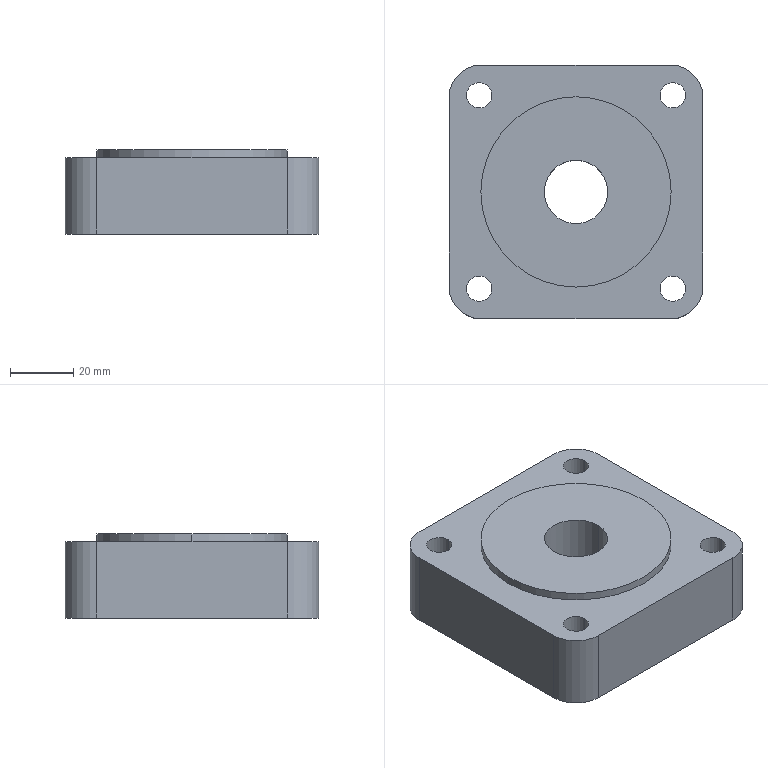Part | SolidWorks | features ICE 4, MirrorPattern 2, Extrusion 1, Fillet 1 | 1 solid | 32 faces | box 80 x 80 x 26.5 mm | volume 139825 mm3 | cylinder 20 | plane 12 | commonest cylinder face diameters 8 x8 20 x6 4 x4 60 x2
STEP:
#1=CARTESIAN_POINT('',(10.,0.,2.5));
#2=VERTEX_POINT('',#1);
#3=CARTESIAN_POINT('',(-10.,0.,2.5));
#4=VERTEX_POINT('',#3);
#5=CARTESIAN_POINT('',(0.,0.,2.5));
#6=DIRECTION('',(0.,0.,-1.));
#7=DIRECTION('',(1.,0.,0.));
#8=AXIS2_PLACEMENT_3D('',#5,#6,#7);
#9=CIRCLE('',#8,10.);
#10=EDGE_CURVE('',#2,#4,#9,.T.);
#11=ORIENTED_EDGE('',*,*,#10,.T.);
#12=CARTESIAN_POINT('',(-10.,0.,26.5));
#13=VERTEX_POINT('',#12);
#14=CARTESIAN_POINT('',(-10.,0.,-23.));
#15=DIRECTION('',(0.,0.,1.));
#16=VECTOR('',#15,1000.);
#17=LINE('',#14,#16);
#18=EDGE_CURVE('',#4,#13,#17,.T.);
#19=ORIENTED_EDGE('',*,*,#18,.T.);
#20=CARTESIAN_POINT('',(10.,0.,26.5));
#21=VERTEX_POINT('',#20);
#22=CARTESIAN_POINT('',(0.,0.,26.5));
#23=DIRECTION('',(0.,0.,1.));
#24=DIRECTION('',(1.,0.,0.));
#25=AXIS2_PLACEMENT_3D('',#22,#23,#24);
#26=CIRCLE('',#25,10.);
#27=EDGE_CURVE('',#13,#21,#26,.T.);
#28=ORIENTED_EDGE('',*,*,#27,.T.);
#29=CARTESIAN_POINT('',(10.,0.,-23.));
#30=DIRECTION('',(0.,0.,1.));
#31=VECTOR('',#30,1000.);
#32=LINE('',#29,#31);
#33=EDGE_CURVE('',#2,#21,#32,.T.);
#34=ORIENTED_EDGE('',*,*,#33,.F.);
#35=EDGE_LOOP('',(#11,#19,#28,#34));
#36=FACE_OUTER_BOUND('',#35,.T.);
#37=CARTESIAN_POINT('',(0.,0.,-23.));
#38=DIRECTION('',(0.,0.,1.));
#39=DIRECTION('',(1.,0.,0.));
#40=AXIS2_PLACEMENT_3D('',#37,#38,#39);
#41=CYLINDRICAL_SURFACE('',#40,10.);
#42=ADVANCED_FACE('',(#36),#41,.F.);
#43=CARTESIAN_POINT('',(30.,0.,26.5));
#44=VERTEX_POINT('',#43);
#45=CARTESIAN_POINT('',(-30.,0.,26.5));
#46=VERTEX_POINT('',#45);
#47=CARTESIAN_POINT('',(0.,0.,26.5));
#48=DIRECTION('',(0.,0.,1.));
#49=DIRECTION('',(1.,0.,0.));
#50=AXIS2_PLACEMENT_3D('',#47,#48,#49);
#51=CIRCLE('',#50,30.);
#52=EDGE_CURVE('',#44,#46,#51,.T.);
#53=ORIENTED_EDGE('',*,*,#52,.F.);
#54=CARTESIAN_POINT('',(30.,0.,24.));
#55=VERTEX_POINT('',#54);
#56=CARTESIAN_POINT('',(30.,0.,26.5));
#57=DIRECTION('',(0.,0.,-1.));
#58=VECTOR('',#57,1000.);
#59=LINE('',#56,#58);
#60=EDGE_CURVE('',#44,#55,#59,.T.);
#61=ORIENTED_EDGE('',*,*,#60,.T.);
#62=CARTESIAN_POINT('',(-30.,0.,24.));
#63=VERTEX_POINT('',#62);
#64=CARTESIAN_POINT('',(0.,0.,24.));
#65=DIRECTION('',(0.,0.,1.));
#66=DIRECTION('',(-1.,0.,0.));
#67=AXIS2_PLACEMENT_3D('',#64,#65,#66);
#68=CIRCLE('',#67,30.);
#69=EDGE_CURVE('',#55,#63,#68,.T.);
#70=ORIENTED_EDGE('',*,*,#69,.T.);
#71=CARTESIAN_POINT('',(-30.,0.,26.5));
#72=DIRECTION('',(0.,0.,-1.));
#73=VECTOR('',#72,1000.);
#74=LINE('',#71,#73);
#75=EDGE_CURVE('',#46,#63,#74,.T.);
#76=ORIENTED_EDGE('',*,*,#75,.F.);
#77=EDGE_LOOP('',(#53,#61,#70,#76));
#78=FACE_OUTER_BOUND('',#77,.T.);
#79=CARTESIAN_POINT('',(0.,0.,26.5));
#80=DIRECTION('',(0.,0.,-1.));
#81=DIRECTION('',(-1.,0.,0.));
#82=AXIS2_PLACEMENT_3D('',#79,#80,#81);
#83=CYLINDRICAL_SURFACE('',#82,30.);
#84=ADVANCED_FACE('',(#78),#83,.T.);
#85=CARTESIAN_POINT('',(34.5,30.5,0.));
#86=VERTEX_POINT('',#85);
#87=CARTESIAN_POINT('',(26.5,30.5,0.));
#88=VERTEX_POINT('',#87);
#89=CARTESIAN_POINT('',(30.5,30.5,0.));
#90=DIRECTION('',(0.,0.,-1.));
#91=DIRECTION('',(-1.,0.,0.));
#92=AXIS2_PLACEMENT_3D('',#89,#90,#91);
#93=CIRCLE('',#92,4.);
#94=EDGE_CURVE('',#86,#88,#93,.T.);
#95=ORIENTED_EDGE('',*,*,#94,.T.);
#96=CARTESIAN_POINT('',(26.5,30.5,24.));
#97=VERTEX_POINT('',#96);
#98=CARTESIAN_POINT('',(26.5,30.5,0.));
#99=DIRECTION('',(0.,0.,1.));
#100=VECTOR('',#99,1000.);
#101=LINE('',#98,#100);
#102=EDGE_CURVE('',#88,#97,#101,.T.);
#103=ORIENTED_EDGE('',*,*,#102,.T.);
#104=CARTESIAN_POINT('',(34.5,30.5,24.));
#105=VERTEX_POINT('',#104);
#106=CARTESIAN_POINT('',(30.5,30.5,24.));
#107=DIRECTION('',(0.,0.,1.));
#108=DIRECTION('',(-1.,0.,0.));
#109=AXIS2_PLACEMENT_3D('',#106,#107,#108);
#110=CIRCLE('',#109,4.);
#111=EDGE_CURVE('',#97,#105,#110,.T.);
#112=ORIENTED_EDGE('',*,*,#111,.T.);
#113=CARTESIAN_POINT('',(34.5,30.5,0.));
#114=DIRECTION('',(0.,0.,1.));
#115=VECTOR('',#114,1000.);
#116=LINE('',#113,#115);
#117=EDGE_CURVE('',#86,#105,#116,.T.);
#118=ORIENTED_EDGE('',*,*,#117,.F.);
#119=EDGE_LOOP('',(#95,#103,#112,#118));
#120=FACE_OUTER_BOUND('',#119,.T.);
#121=CARTESIAN_POINT('',(30.5,30.5,0.));
#122=DIRECTION('',(0.,0.,1.));
#123=DIRECTION('',(1.,0.,0.));
#124=AXIS2_PLACEMENT_3D('',#121,#122,#123);
#125=CYLINDRICAL_SURFACE('',#124,4.);
#126=ADVANCED_FACE('',(#120),#125,.F.);
#127=CARTESIAN_POINT('',(26.5,-30.5,0.));
#128=VERTEX_POINT('',#127);
#129=CARTESIAN_POINT('',(34.5,-30.5,0.));
#130=VERTEX_POINT('',#129);
#131=CARTESIAN_POINT('',(30.5,-30.5,0.));
#132=DIRECTION('',(0.,0.,1.));
#133=DIRECTION('',(-1.,0.,0.));
#134=AXIS2_PLACEMENT_3D('',#131,#132,#133);
#135=CIRCLE('',#134,4.);
#136=EDGE_CURVE('',#128,#130,#135,.T.);
#137=ORIENTED_EDGE('',*,*,#136,.F.);
#138=CARTESIAN_POINT('',(26.5,-30.5,24.));
#139=VERTEX_POINT('',#138);
#140=CARTESIAN_POINT('',(26.5,-30.5,0.));
#141=DIRECTION('',(0.,0.,1.));
#142=VECTOR('',#141,1000.);
#143=LINE('',#140,#142);
#144=EDGE_CURVE('',#128,#139,#143,.T.);
#145=ORIENTED_EDGE('',*,*,#144,.T.);
#146=CARTESIAN_POINT('',(34.5,-30.5,24.));
#147=VERTEX_POINT('',#146);
#148=CARTESIAN_POINT('',(30.5,-30.5,24.));
#149=DIRECTION('',(0.,0.,-1.));
#150=DIRECTION('',(-1.,0.,0.));
#151=AXIS2_PLACEMENT_3D('',#148,#149,#150);
#152=CIRCLE('',#151,4.);
#153=EDGE_CURVE('',#147,#139,#152,.T.);
#154=ORIENTED_EDGE('',*,*,#153,.F.);
#155=CARTESIAN_POINT('',(34.5,-30.5,0.));
#156=DIRECTION('',(0.,0.,1.));
#157=VECTOR('',#156,1000.);
#158=LINE('',#155,#157);
#159=EDGE_CURVE('',#130,#147,#158,.T.);
#160=ORIENTED_EDGE('',*,*,#159,.F.);
#161=EDGE_LOOP('',(#137,#145,#154,#160));
#162=FACE_OUTER_BOUND('',#161,.T.);
#163=CARTESIAN_POINT('',(30.5,-30.5,0.));
#164=DIRECTION('',(0.,0.,1.));
#165=DIRECTION('',(1.,0.,0.));
#166=AXIS2_PLACEMENT_3D('',#163,#164,#165);
#167=CYLINDRICAL_SURFACE('',#166,4.);
#168=ADVANCED_FACE('',(#162),#167,.F.);
#169=CARTESIAN_POINT('',(-26.5,-30.5,0.));
#170=VERTEX_POINT('',#169);
#171=CARTESIAN_POINT('',(-34.5,-30.5,0.));
#172=VERTEX_POINT('',#171);
#173=CARTESIAN_POINT('',(-30.5,-30.5,0.));
#174=DIRECTION('',(0.,0.,-1.));
#175=DIRECTION('',(1.,0.,0.));
#176=AXIS2_PLACEMENT_3D('',#173,#174,#175);
#177=CIRCLE('',#176,4.);
#178=EDGE_CURVE('',#170,#172,#177,.T.);
#179=ORIENTED_EDGE('',*,*,#178,.T.);
#180=CARTESIAN_POINT('',(-34.5,-30.5,24.));
#181=VERTEX_POINT('',#180);
#182=CARTESIAN_POINT('',(-34.5,-30.5,0.));
#183=DIRECTION('',(0.,0.,1.));
#184=VECTOR('',#183,1000.);
#185=LINE('',#182,#184);
#186=EDGE_CURVE('',#172,#181,#185,.T.);
#187=ORIENTED_EDGE('',*,*,#186,.T.);
#188=CARTESIAN_POINT('',(-26.5,-30.5,24.));
#189=VERTEX_POINT('',#188);
#190=CARTESIAN_POINT('',(-30.5,-30.5,24.));
#191=DIRECTION('',(0.,0.,1.));
#192=DIRECTION('',(-1.,0.,0.));
#193=AXIS2_PLACEMENT_3D('',#190,#191,#192);
#194=CIRCLE('',#193,4.);
#195=EDGE_CURVE('',#181,#189,#194,.T.);
#196=ORIENTED_EDGE('',*,*,#195,.T.);
#197=CARTESIAN_POINT('',(-26.5,-30.5,0.));
#198=DIRECTION('',(0.,0.,1.));
#199=VECTOR('',#198,1000.);
#200=LINE('',#197,#199);
#201=EDGE_CURVE('',#170,#189,#200,.T.);
#202=ORIENTED_EDGE('',*,*,#201,.F.);
#203=EDGE_LOOP('',(#179,#187,#196,#202));
#204=FACE_OUTER_BOUND('',#203,.T.);
#205=CARTESIAN_POINT('',(-30.5,-30.5,0.));
#206=DIRECTION('',(0.,0.,1.));
#207=DIRECTION('',(1.,0.,0.));
#208=AXIS2_PLACEMENT_3D('',#205,#206,#207);
#209=CYLINDRICAL_SURFACE('',#208,4.);
#210=ADVANCED_FACE('',(#204),#209,.F.);
#211=CARTESIAN_POINT('',(-34.5,30.5,0.));
#212=VERTEX_POINT('',#211);
#213=CARTESIAN_POINT('',(-26.5,30.5,0.));
#214=VERTEX_POINT('',#213);
#215=CARTESIAN_POINT('',(-30.5,30.5,0.));
#216=DIRECTION('',(0.,0.,1.));
#217=DIRECTION('',(1.,0.,0.));
#218=AXIS2_PLACEMENT_3D('',#215,#216,#217);
#219=CIRCLE('',#218,4.);
#220=EDGE_CURVE('',#212,#214,#219,.T.);
#221=ORIENTED_EDGE('',*,*,#220,.F.);
#222=CARTESIAN_POINT('',(-34.5,30.5,24.));
#223=VERTEX_POINT('',#222);
#224=CARTESIAN_POINT('',(-34.5,30.5,0.));
#225=DIRECTION('',(0.,0.,1.));
#226=VECTOR('',#225,1000.);
#227=LINE('',#224,#226);
#228=EDGE_CURVE('',#212,#223,#227,.T.);
#229=ORIENTED_EDGE('',*,*,#228,.T.);
#230=CARTESIAN_POINT('',(-26.5,30.5,24.));
#231=VERTEX_POINT('',#230);
#232=CARTESIAN_POINT('',(-30.5,30.5,24.));
#233=DIRECTION('',(0.,0.,-1.));
#234=DIRECTION('',(-1.,0.,0.));
#235=AXIS2_PLACEMENT_3D('',#232,#233,#234);
#236=CIRCLE('',#235,4.);
#237=EDGE_CURVE('',#231,#223,#236,.T.);
#238=ORIENTED_EDGE('',*,*,#237,.F.);
#239=CARTESIAN_POINT('',(-26.5,30.5,0.));
#240=DIRECTION('',(0.,0.,1.));
#241=VECTOR('',#240,1000.);
#242=LINE('',#239,#241);
#243=EDGE_CURVE('',#214,#231,#242,.T.);
#244=ORIENTED_EDGE('',*,*,#243,.F.);
#245=EDGE_LOOP('',(#221,#229,#238,#244));
#246=FACE_OUTER_BOUND('',#245,.T.);
#247=CARTESIAN_POINT('',(-30.5,30.5,0.));
#248=DIRECTION('',(0.,0.,1.));
#249=DIRECTION('',(1.,0.,0.));
#250=AXIS2_PLACEMENT_3D('',#247,#248,#249);
#251=CYLINDRICAL_SURFACE('',#250,4.);
#252=ADVANCED_FACE('',(#246),#251,.F.);
#253=CARTESIAN_POINT('',(40.,-30.,24.));
#254=VERTEX_POINT('',#253);
#255=CARTESIAN_POINT('',(40.,30.,24.));
#256=VERTEX_POINT('',#255);
#257=CARTESIAN_POINT('',(40.,-40.,24.));
#258=DIRECTION('',(0.,1.,0.));
#259=VECTOR('',#258,1000.);
#260=LINE('',#257,#259);
#261=EDGE_CURVE('',#254,#256,#260,.T.);
#262=ORIENTED_EDGE('',*,*,#261,.F.);
#263=CARTESIAN_POINT('',(40.,-30.,0.));
#264=VERTEX_POINT('',#263);
#265=CARTESIAN_POINT('',(40.,-30.,24.));
#266=DIRECTION('',(0.,0.,-1.));
#267=VECTOR('',#266,1000.);
#268=LINE('',#265,#267);
#269=EDGE_CURVE('',#254,#264,#268,.T.);
#270=ORIENTED_EDGE('',*,*,#269,.T.);
#271=CARTESIAN_POINT('',(40.,30.,0.));
#272=VERTEX_POINT('',#271);
#273=CARTESIAN_POINT('',(40.,-40.,0.));
#274=DIRECTION('',(0.,1.,0.));
#275=VECTOR('',#274,1000.);
#276=LINE('',#273,#275);
#277=EDGE_CURVE('',#264,#272,#276,.T.);
#278=ORIENTED_EDGE('',*,*,#277,.T.);
#279=CARTESIAN_POINT('',(40.,30.,24.));
#280=DIRECTION('',(0.,0.,1.));
#281=VECTOR('',#280,1000.);
#282=LINE('',#279,#281);
#283=EDGE_CURVE('',#272,#256,#282,.T.);
#284=ORIENTED_EDGE('',*,*,#283,.T.);
#285=EDGE_LOOP('',(#262,#270,#278,#284));
#286=FACE_OUTER_BOUND('',#285,.T.);
#287=CARTESIAN_POINT('',(40.,-40.,24.));
#288=DIRECTION('',(-1.,0.,0.));
#289=DIRECTION('',(0.,0.,1.));
#290=AXIS2_PLACEMENT_3D('',#287,#288,#289);
#291=PLANE('',#290);
#292=ADVANCED_FACE('',(#286),#291,.F.);
#293=CARTESIAN_POINT('',(30.,40.,24.));
#294=VERTEX_POINT('',#293);
#295=CARTESIAN_POINT('',(-30.,40.,24.));
#296=VERTEX_POINT('',#295);
#297=CARTESIAN_POINT('',(-40.,40.,24.));
#298=DIRECTION('',(-1.,0.,0.));
#299=VECTOR('',#298,1000.);
#300=LINE('',#297,#299);
#301=EDGE_CURVE('',#294,#296,#300,.T.);
#302=ORIENTED_EDGE('',*,*,#301,.F.);
#303=CARTESIAN_POINT('',(30.,40.,0.));
#304=VERTEX_POINT('',#303);
#305=CARTESIAN_POINT('',(30.,40.,24.));
#306=DIRECTION('',(0.,0.,-1.));
#307=VECTOR('',#306,1000.);
#308=LINE('',#305,#307);
#309=EDGE_CURVE('',#294,#304,#308,.T.);
#310=ORIENTED_EDGE('',*,*,#309,.T.);
#311=CARTESIAN_POINT('',(-30.,40.,0.));
#312=VERTEX_POINT('',#311);
#313=CARTESIAN_POINT('',(-40.,40.,0.));
#314=DIRECTION('',(-1.,0.,0.));
#315=VECTOR('',#314,1000.);
#316=LINE('',#313,#315);
#317=EDGE_CURVE('',#304,#312,#316,.T.);
#318=ORIENTED_EDGE('',*,*,#317,.T.);
#319=CARTESIAN_POINT('',(-30.,40.,24.));
#320=DIRECTION('',(0.,0.,1.));
#321=VECTOR('',#320,1000.);
#322=LINE('',#319,#321);
#323=EDGE_CURVE('',#312,#296,#322,.T.);
#324=ORIENTED_EDGE('',*,*,#323,.T.);
#325=EDGE_LOOP('',(#302,#310,#318,#324));
#326=FACE_OUTER_BOUND('',#325,.T.);
#327=CARTESIAN_POINT('',(-40.,40.,24.));
#328=DIRECTION('',(0.,-1.,0.));
#329=DIRECTION('',(0.,0.,-1.));
#330=AXIS2_PLACEMENT_3D('',#327,#328,#329);
#331=PLANE('',#330);
#332=ADVANCED_FACE('',(#326),#331,.F.);
#333=CARTESIAN_POINT('',(-40.,30.,0.));
#334=VERTEX_POINT('',#333);
#335=CARTESIAN_POINT('',(-40.,-30.,0.));
#336=VERTEX_POINT('',#335);
#337=CARTESIAN_POINT('',(-40.,-40.,0.));
#338=DIRECTION('',(0.,-1.,0.));
#339=VECTOR('',#338,1000.);
#340=LINE('',#337,#339);
#341=EDGE_CURVE('',#334,#336,#340,.T.);
#342=ORIENTED_EDGE('',*,*,#341,.T.);
#343=CARTESIAN_POINT('',(-40.,-30.,24.));
#344=VERTEX_POINT('',#343);
#345=CARTESIAN_POINT('',(-40.,-30.,24.));
#346=DIRECTION('',(0.,0.,1.));
#347=VECTOR('',#346,1000.);
#348=LINE('',#345,#347);
#349=EDGE_CURVE('',#336,#344,#348,.T.);
#350=ORIENTED_EDGE('',*,*,#349,.T.);
#351=CARTESIAN_POINT('',(-40.,30.,24.));
#352=VERTEX_POINT('',#351);
#353=CARTESIAN_POINT('',(-40.,-40.,24.));
#354=DIRECTION('',(0.,-1.,0.));
#355=VECTOR('',#354,1000.);
#356=LINE('',#353,#355);
#357=EDGE_CURVE('',#352,#344,#356,.T.);
#358=ORIENTED_EDGE('',*,*,#357,.F.);
#359=CARTESIAN_POINT('',(-40.,30.,24.));
#360=DIRECTION('',(0.,0.,-1.));
#361=VECTOR('',#360,1000.);
#362=LINE('',#359,#361);
#363=EDGE_CURVE('',#352,#334,#362,.T.);
#364=ORIENTED_EDGE('',*,*,#363,.T.);
#365=EDGE_LOOP('',(#342,#350,#358,#364));
#366=FACE_OUTER_BOUND('',#365,.T.);
#367=CARTESIAN_POINT('',(-40.,-40.,24.));
#368=DIRECTION('',(1.,0.,0.));
#369=DIRECTION('',(0.,0.,-1.));
#370=AXIS2_PLACEMENT_3D('',#367,#368,#369);
#371=PLANE('',#370);
#372=ADVANCED_FACE('',(#366),#371,.F.);
#373=CARTESIAN_POINT('',(-30.,-40.,24.));
#374=VERTEX_POINT('',#373);
#375=CARTESIAN_POINT('',(30.,-40.,24.));
#376=VERTEX_POINT('',#375);
#377=CARTESIAN_POINT('',(-40.,-40.,24.));
#378=DIRECTION('',(1.,0.,0.));
#379=VECTOR('',#378,1000.);
#380=LINE('',#377,#379);
#381=EDGE_CURVE('',#374,#376,#380,.T.);
#382=ORIENTED_EDGE('',*,*,#381,.F.);
#383=CARTESIAN_POINT('',(-30.,-40.,0.));
#384=VERTEX_POINT('',#383);
#385=CARTESIAN_POINT('',(-30.,-40.,24.));
#386=DIRECTION('',(0.,0.,-1.));
#387=VECTOR('',#386,1000.);
#388=LINE('',#385,#387);
#389=EDGE_CURVE('',#374,#384,#388,.T.);
#390=ORIENTED_EDGE('',*,*,#389,.T.);
#391=CARTESIAN_POINT('',(30.,-40.,0.));
#392=VERTEX_POINT('',#391);
#393=CARTESIAN_POINT('',(-40.,-40.,0.));
#394=DIRECTION('',(1.,0.,0.));
#395=VECTOR('',#394,1000.);
#396=LINE('',#393,#395);
#397=EDGE_CURVE('',#384,#392,#396,.T.);
#398=ORIENTED_EDGE('',*,*,#397,.T.);
#399=CARTESIAN_POINT('',(30.,-40.,24.));
#400=DIRECTION('',(0.,0.,1.));
#401=VECTOR('',#400,1000.);
#402=LINE('',#399,#401);
#403=EDGE_CURVE('',#392,#376,#402,.T.);
#404=ORIENTED_EDGE('',*,*,#403,.T.);
#405=EDGE_LOOP('',(#382,#390,#398,#404));
#406=FACE_OUTER_BOUND('',#405,.T.);
#407=CARTESIAN_POINT('',(-40.,-40.,24.));
#408=DIRECTION('',(0.,1.,0.));
#409=DIRECTION('',(0.,0.,1.));
#410=AXIS2_PLACEMENT_3D('',#407,#408,#409);
#411=PLANE('',#410);
#412=ADVANCED_FACE('',(#406),#411,.F.);
#413=CARTESIAN_POINT('',(0.,0.,24.));
#414=DIRECTION('',(0.,0.,1.));
#415=DIRECTION('',(-1.,0.,0.));
#416=AXIS2_PLACEMENT_3D('',#413,#414,#415);
#417=CIRCLE('',#416,30.);
#418=EDGE_CURVE('',#63,#55,#417,.T.);
#419=ORIENTED_EDGE('',*,*,#418,.F.);
#420=ORIENTED_EDGE('',*,*,#69,.F.);
#421=EDGE_LOOP('',(#419,#420));
#422=FACE_BOUND('',#421,.T.);
#423=CARTESIAN_POINT('',(30.5,30.5,24.));
#424=DIRECTION('',(0.,0.,1.));
#425=DIRECTION('',(-1.,0.,0.));
#426=AXIS2_PLACEMENT_3D('',#423,#424,#425);
#427=CIRCLE('',#426,4.);
#428=EDGE_CURVE('',#105,#97,#427,.T.);
#429=ORIENTED_EDGE('',*,*,#428,.F.);
#430=ORIENTED_EDGE('',*,*,#111,.F.);
#431=EDGE_LOOP('',(#429,#430));
#432=FACE_BOUND('',#431,.T.);
#433=ORIENTED_EDGE('',*,*,#153,.T.);
#434=CARTESIAN_POINT('',(30.5,-30.5,24.));
#435=DIRECTION('',(0.,0.,-1.));
#436=DIRECTION('',(-1.,0.,0.));
#437=AXIS2_PLACEMENT_3D('',#434,#435,#436);
#438=CIRCLE('',#437,4.);
#439=EDGE_CURVE('',#139,#147,#438,.T.);
#440=ORIENTED_EDGE('',*,*,#439,.T.);
#441=EDGE_LOOP('',(#433,#440));
#442=FACE_BOUND('',#441,.T.);
#443=CARTESIAN_POINT('',(-30.5,-30.5,24.));
#444=DIRECTION('',(0.,0.,1.));
#445=DIRECTION('',(-1.,0.,0.));
#446=AXIS2_PLACEMENT_3D('',#443,#444,#445);
#447=CIRCLE('',#446,4.);
#448=EDGE_CURVE('',#189,#181,#447,.T.);
#449=ORIENTED_EDGE('',*,*,#448,.F.);
#450=ORIENTED_EDGE('',*,*,#195,.F.);
#451=EDGE_LOOP('',(#449,#450));
#452=FACE_BOUND('',#451,.T.);
#453=ORIENTED_EDGE('',*,*,#237,.T.);
#454=CARTESIAN_POINT('',(-30.5,30.5,24.));
#455=DIRECTION('',(0.,0.,-1.));
#456=DIRECTION('',(-1.,0.,0.));
#457=AXIS2_PLACEMENT_3D('',#454,#455,#456);
#458=CIRCLE('',#457,4.);
#459=EDGE_CURVE('',#223,#231,#458,.T.);
#460=ORIENTED_EDGE('',*,*,#459,.T.);
#461=EDGE_LOOP('',(#453,#460));
#462=FACE_BOUND('',#461,.T.);
#463=ORIENTED_EDGE('',*,*,#357,.T.);
#464=CARTESIAN_POINT('',(-30.,-30.,24.));
#465=DIRECTION('',(0.,0.,1.));
#466=DIRECTION('',(-1.,0.,0.));
#467=AXIS2_PLACEMENT_3D('',#464,#465,#466);
#468=CIRCLE('',#467,10.);
#469=EDGE_CURVE('',#344,#374,#468,.T.);
#470=ORIENTED_EDGE('',*,*,#469,.T.);
#471=ORIENTED_EDGE('',*,*,#381,.T.);
#472=CARTESIAN_POINT('',(30.,-30.,24.));
#473=DIRECTION('',(0.,0.,1.));
#474=DIRECTION('',(-1.,0.,0.));
#475=AXIS2_PLACEMENT_3D('',#472,#473,#474);
#476=CIRCLE('',#475,10.);
#477=EDGE_CURVE('',#376,#254,#476,.T.);
#478=ORIENTED_EDGE('',*,*,#477,.T.);
#479=ORIENTED_EDGE('',*,*,#261,.T.);
#480=CARTESIAN_POINT('',(30.,30.,24.));
#481=DIRECTION('',(0.,0.,1.));
#482=DIRECTION('',(-1.,0.,0.));
#483=AXIS2_PLACEMENT_3D('',#480,#481,#482);
#484=CIRCLE('',#483,10.);
#485=EDGE_CURVE('',#256,#294,#484,.T.);
#486=ORIENTED_EDGE('',*,*,#485,.T.);
#487=ORIENTED_EDGE('',*,*,#301,.T.);
#488=CARTESIAN_POINT('',(-30.,30.,24.));
#489=DIRECTION('',(0.,0.,1.));
#490=DIRECTION('',(-1.,0.,0.));
#491=AXIS2_PLACEMENT_3D('',#488,#489,#490);
#492=CIRCLE('',#491,10.);
#493=EDGE_CURVE('',#296,#352,#492,.T.);
#494=ORIENTED_EDGE('',*,*,#493,.T.);
#495=EDGE_LOOP('',(#463,#470,#471,#478,#479,#486,#487,#494));
#496=FACE_OUTER_BOUND('',#495,.T.);
#497=CARTESIAN_POINT('',(0.,0.,24.));
#498=DIRECTION('',(0.,0.,-1.));
#499=DIRECTION('',(-1.,0.,0.));
#500=AXIS2_PLACEMENT_3D('',#497,#498,#499);
#501=PLANE('',#500);
#502=ADVANCED_FACE('',(#422,#432,#442,#452,#462,#496),#501,.F.);
#503=CARTESIAN_POINT('',(25.263,-23.439,0.));
#504=VERTEX_POINT('',#503);
#505=CARTESIAN_POINT('',(23.263,-25.439,0.));
#506=VERTEX_POINT('',#505);
#507=CARTESIAN_POINT('',(23.263,-23.439,0.));
#508=DIRECTION('',(0.,0.,-1.));
#509=DIRECTION('',(1.,0.,0.));
#510=AXIS2_PLACEMENT_3D('',#507,#508,#509);
#511=CIRCLE('',#510,2.);
#512=EDGE_CURVE('',#504,#506,#511,.T.);
#513=ORIENTED_EDGE('',*,*,#512,.F.);
#514=CARTESIAN_POINT('',(25.263,23.439,0.));
#515=VERTEX_POINT('',#514);
#516=CARTESIAN_POINT('',(25.263,-23.439,0.));
#517=DIRECTION('',(0.,-1.,0.));
#518=VECTOR('',#517,1000.);
#519=LINE('',#516,#518);
#520=EDGE_CURVE('',#515,#504,#519,.T.);
#521=ORIENTED_EDGE('',*,*,#520,.F.);
#522=CARTESIAN_POINT('',(23.263,25.439,0.));
#523=VERTEX_POINT('',#522);
#524=CARTESIAN_POINT('',(23.263,23.439,0.));
#525=DIRECTION('',(0.,0.,-1.));
#526=DIRECTION('',(1.,0.,0.));
#527=AXIS2_PLACEMENT_3D('',#524,#525,#526);
#528=CIRCLE('',#527,2.);
#529=EDGE_CURVE('',#523,#515,#528,.T.);
#530=ORIENTED_EDGE('',*,*,#529,.F.);
#531=CARTESIAN_POINT('',(-23.263,25.439,0.));
#532=VERTEX_POINT('',#531);
#533=CARTESIAN_POINT('',(23.263,25.439,0.));
#534=DIRECTION('',(1.,0.,0.));
#535=VECTOR('',#534,1000.);
#536=LINE('',#533,#535);
#537=EDGE_CURVE('',#532,#523,#536,.T.);
#538=ORIENTED_EDGE('',*,*,#537,.F.);
#539=CARTESIAN_POINT('',(-25.263,23.439,0.));
#540=VERTEX_POINT('',#539);
#541=CARTESIAN_POINT('',(-23.263,23.439,0.));
#542=DIRECTION('',(0.,0.,-1.));
#543=DIRECTION('',(-1.,0.,0.));
#544=AXIS2_PLACEMENT_3D('',#541,#542,#543);
#545=CIRCLE('',#544,2.);
#546=EDGE_CURVE('',#540,#532,#545,.T.);
#547=ORIENTED_EDGE('',*,*,#546,.F.);
#548=CARTESIAN_POINT('',(-25.263,-23.439,0.));
#549=VERTEX_POINT('',#548);
#550=CARTESIAN_POINT('',(-25.263,-23.439,0.));
#551=DIRECTION('',(0.,1.,0.));
#552=VECTOR('',#551,1000.);
#553=LINE('',#550,#552);
#554=EDGE_CURVE('',#549,#540,#553,.T.);
#555=ORIENTED_EDGE('',*,*,#554,.F.);
#556=CARTESIAN_POINT('',(-23.263,-25.439,0.));
#557=VERTEX_POINT('',#556);
#558=CARTESIAN_POINT('',(-23.263,-23.439,0.));
#559=DIRECTION('',(0.,0.,-1.));
#560=DIRECTION('',(1.,0.,0.));
#561=AXIS2_PLACEMENT_3D('',#558,#559,#560);
#562=CIRCLE('',#561,2.);
#563=EDGE_CURVE('',#557,#549,#562,.T.);
#564=ORIENTED_EDGE('',*,*,#563,.F.);
#565=CARTESIAN_POINT('',(23.263,-25.439,0.));
#566=DIRECTION('',(-1.,0.,0.));
#567=VECTOR('',#566,1000.);
#568=LINE('',#565,#567);
#569=EDGE_CURVE('',#506,#557,#568,.T.);
#570=ORIENTED_EDGE('',*,*,#569,.F.);
#571=EDGE_LOOP('',(#513,#521,#530,#538,#547,#555,#564,#570));
#572=FACE_BOUND('',#571,.T.);
#573=ORIENTED_EDGE('',*,*,#94,.F.);
#574=CARTESIAN_POINT('',(30.5,30.5,0.));
#575=DIRECTION('',(0.,0.,-1.));
#576=DIRECTION('',(-1.,0.,0.));
#577=AXIS2_PLACEMENT_3D('',#574,#575,#576);
#578=CIRCLE('',#577,4.);
#579=EDGE_CURVE('',#88,#86,#578,.T.);
#580=ORIENTED_EDGE('',*,*,#579,.F.);
#581=EDGE_LOOP('',(#573,#580));
#582=FACE_BOUND('',#581,.T.);
#583=CARTESIAN_POINT('',(30.5,-30.5,0.));
#584=DIRECTION('',(0.,0.,1.));
#585=DIRECTION('',(-1.,0.,0.));
#586=AXIS2_PLACEMENT_3D('',#583,#584,#585);
#587=CIRCLE('',#586,4.);
#588=EDGE_CURVE('',#130,#128,#587,.T.);
#589=ORIENTED_EDGE('',*,*,#588,.T.);
#590=ORIENTED_EDGE('',*,*,#136,.T.);
#591=EDGE_LOOP('',(#589,#590));
#592=FACE_BOUND('',#591,.T.);
#593=ORIENTED_EDGE('',*,*,#178,.F.);
#594=CARTESIAN_POINT('',(-30.5,-30.5,0.));
#595=DIRECTION('',(0.,0.,-1.));
#596=DIRECTION('',(1.,0.,0.));
#597=AXIS2_PLACEMENT_3D('',#594,#595,#596);
#598=CIRCLE('',#597,4.);
#599=EDGE_CURVE('',#172,#170,#598,.T.);
#600=ORIENTED_EDGE('',*,*,#599,.F.);
#601=EDGE_LOOP('',(#593,#600));
#602=FACE_BOUND('',#601,.T.);
#603=CARTESIAN_POINT('',(-30.5,30.5,0.));
#604=DIRECTION('',(0.,0.,1.));
#605=DIRECTION('',(1.,0.,0.));
#606=AXIS2_PLACEMENT_3D('',#603,#604,#605);
#607=CIRCLE('',#606,4.);
#608=EDGE_CURVE('',#214,#212,#607,.T.);
#609=ORIENTED_EDGE('',*,*,#608,.T.);
#610=ORIENTED_EDGE('',*,*,#220,.T.);
#611=EDGE_LOOP('',(#609,#610));
#612=FACE_BOUND('',#611,.T.);
#613=ORIENTED_EDGE('',*,*,#397,.F.);
#614=CARTESIAN_POINT('',(-30.,-30.,0.));
#615=DIRECTION('',(0.,0.,-1.));
#616=DIRECTION('',(-1.,0.,0.));
#617=AXIS2_PLACEMENT_3D('',#614,#615,#616);
#618=CIRCLE('',#617,10.);
#619=EDGE_CURVE('',#384,#336,#618,.T.);
#620=ORIENTED_EDGE('',*,*,#619,.T.);
#621=ORIENTED_EDGE('',*,*,#341,.F.);
#622=CARTESIAN_POINT('',(-30.,30.,0.));
#623=DIRECTION('',(0.,0.,-1.));
#624=DIRECTION('',(-1.,0.,0.));
#625=AXIS2_PLACEMENT_3D('',#622,#623,#624);
#626=CIRCLE('',#625,10.);
#627=EDGE_CURVE('',#334,#312,#626,.T.);
#628=ORIENTED_EDGE('',*,*,#627,.T.);
#629=ORIENTED_EDGE('',*,*,#317,.F.);
#630=CARTESIAN_POINT('',(30.,30.,0.));
#631=DIRECTION('',(0.,0.,-1.));
#632=DIRECTION('',(-1.,0.,0.));
#633=AXIS2_PLACEMENT_3D('',#630,#631,#632);
#634=CIRCLE('',#633,10.);
#635=EDGE_CURVE('',#304,#272,#634,.T.);
#636=ORIENTED_EDGE('',*,*,#635,.T.);
#637=ORIENTED_EDGE('',*,*,#277,.F.);
#638=CARTESIAN_POINT('',(30.,-30.,0.));
#639=DIRECTION('',(0.,0.,-1.));
#640=DIRECTION('',(-1.,0.,0.));
#641=AXIS2_PLACEMENT_3D('',#638,#639,#640);
#642=CIRCLE('',#641,10.);
#643=EDGE_CURVE('',#264,#392,#642,.T.);
#644=ORIENTED_EDGE('',*,*,#643,.T.);
#645=EDGE_LOOP('',(#613,#620,#621,#628,#629,#636,#637,#644));
#646=FACE_OUTER_BOUND('',#645,.T.);
#647=CARTESIAN_POINT('',(0.,0.,0.));
#648=DIRECTION('',(0.,0.,-1.));
#649=DIRECTION('',(-1.,0.,0.));
#650=AXIS2_PLACEMENT_3D('',#647,#648,#649);
#651=PLANE('',#650);
#652=ADVANCED_FACE('',(#572,#582,#592,#602,#612,#646),#651,.T.);
#653=ORIENTED_EDGE('',*,*,#469,.F.);
#654=ORIENTED_EDGE('',*,*,#349,.F.);
#655=ORIENTED_EDGE('',*,*,#619,.F.);
#656=ORIENTED_EDGE('',*,*,#389,.F.);
#657=EDGE_LOOP('',(#653,#654,#655,#656));
#658=FACE_OUTER_BOUND('',#657,.T.);
#659=CARTESIAN_POINT('',(-30.,-30.,24.));
#660=DIRECTION('',(0.,0.,-1.));
#661=DIRECTION('',(-1.,0.,0.));
#662=AXIS2_PLACEMENT_3D('',#659,#660,#661);
#663=CYLINDRICAL_SURFACE('',#662,10.);
#664=ADVANCED_FACE('',(#658),#663,.T.);
#665=ORIENTED_EDGE('',*,*,#477,.F.);
#666=ORIENTED_EDGE('',*,*,#403,.F.);
#667=ORIENTED_EDGE('',*,*,#643,.F.);
#668=ORIENTED_EDGE('',*,*,#269,.F.);
#669=EDGE_LOOP('',(#665,#666,#667,#668));
#670=FACE_OUTER_BOUND('',#669,.T.);
#671=CARTESIAN_POINT('',(30.,-30.,24.));
#672=DIRECTION('',(0.,0.,-1.));
#673=DIRECTION('',(-1.,0.,0.));
#674=AXIS2_PLACEMENT_3D('',#671,#672,#673);
#675=CYLINDRICAL_SURFACE('',#674,10.);
#676=ADVANCED_FACE('',(#670),#675,.T.);
#677=ORIENTED_EDGE('',*,*,#485,.F.);
#678=ORIENTED_EDGE('',*,*,#283,.F.);
#679=ORIENTED_EDGE('',*,*,#635,.F.);
#680=ORIENTED_EDGE('',*,*,#309,.F.);
#681=EDGE_LOOP('',(#677,#678,#679,#680));
#682=FACE_OUTER_BOUND('',#681,.T.);
#683=CARTESIAN_POINT('',(30.,30.,24.));
#684=DIRECTION('',(0.,0.,-1.));
#685=DIRECTION('',(-1.,0.,0.));
#686=AXIS2_PLACEMENT_3D('',#683,#684,#685);
#687=CYLINDRICAL_SURFACE('',#686,10.);
#688=ADVANCED_FACE('',(#682),#687,.T.);
#689=ORIENTED_EDGE('',*,*,#493,.F.);
#690=ORIENTED_EDGE('',*,*,#323,.F.);
#691=ORIENTED_EDGE('',*,*,#627,.F.);
#692=ORIENTED_EDGE('',*,*,#363,.F.);
#693=EDGE_LOOP('',(#689,#690,#691,#692));
#694=FACE_OUTER_BOUND('',#693,.T.);
#695=CARTESIAN_POINT('',(-30.,30.,24.));
#696=DIRECTION('',(0.,0.,-1.));
#697=DIRECTION('',(-1.,0.,0.));
#698=AXIS2_PLACEMENT_3D('',#695,#696,#697);
#699=CYLINDRICAL_SURFACE('',#698,10.);
#700=ADVANCED_FACE('',(#694),#699,.T.);
#701=ORIENTED_EDGE('',*,*,#228,.F.);
#702=ORIENTED_EDGE('',*,*,#608,.F.);
#703=ORIENTED_EDGE('',*,*,#243,.T.);
#704=ORIENTED_EDGE('',*,*,#459,.F.);
#705=EDGE_LOOP('',(#701,#702,#703,#704));
#706=FACE_OUTER_BOUND('',#705,.T.);
#707=CARTESIAN_POINT('',(-30.5,30.5,0.));
#708=DIRECTION('',(0.,0.,1.));
#709=DIRECTION('',(1.,0.,0.));
#710=AXIS2_PLACEMENT_3D('',#707,#708,#709);
#711=CYLINDRICAL_SURFACE('',#710,4.);
#712=ADVANCED_FACE('',(#706),#711,.F.);
#713=ORIENTED_EDGE('',*,*,#186,.F.);
#714=ORIENTED_EDGE('',*,*,#599,.T.);
#715=ORIENTED_EDGE('',*,*,#201,.T.);
#716=ORIENTED_EDGE('',*,*,#448,.T.);
#717=EDGE_LOOP('',(#713,#714,#715,#716));
#718=FACE_OUTER_BOUND('',#717,.T.);
#719=CARTESIAN_POINT('',(-30.5,-30.5,0.));
#720=DIRECTION('',(0.,0.,1.));
#721=DIRECTION('',(1.,0.,0.));
#722=AXIS2_PLACEMENT_3D('',#719,#720,#721);
#723=CYLINDRICAL_SURFACE('',#722,4.);
#724=ADVANCED_FACE('',(#718),#723,.F.);
#725=ORIENTED_EDGE('',*,*,#144,.F.);
#726=ORIENTED_EDGE('',*,*,#588,.F.);
#727=ORIENTED_EDGE('',*,*,#159,.T.);
#728=ORIENTED_EDGE('',*,*,#439,.F.);
#729=EDGE_LOOP('',(#725,#726,#727,#728));
#730=FACE_OUTER_BOUND('',#729,.T.);
#731=CARTESIAN_POINT('',(30.5,-30.5,0.));
#732=DIRECTION('',(0.,0.,1.));
#733=DIRECTION('',(1.,0.,0.));
#734=AXIS2_PLACEMENT_3D('',#731,#732,#733);
#735=CYLINDRICAL_SURFACE('',#734,4.);
#736=ADVANCED_FACE('',(#730),#735,.F.);
#737=ORIENTED_EDGE('',*,*,#102,.F.);
#738=ORIENTED_EDGE('',*,*,#579,.T.);
#739=ORIENTED_EDGE('',*,*,#117,.T.);
#740=ORIENTED_EDGE('',*,*,#428,.T.);
#741=EDGE_LOOP('',(#737,#738,#739,#740));
#742=FACE_OUTER_BOUND('',#741,.T.);
#743=CARTESIAN_POINT('',(30.5,30.5,0.));
#744=DIRECTION('',(0.,0.,1.));
#745=DIRECTION('',(1.,0.,0.));
#746=AXIS2_PLACEMENT_3D('',#743,#744,#745);
#747=CYLINDRICAL_SURFACE('',#746,4.);
#748=ADVANCED_FACE('',(#742),#747,.F.);
#749=ORIENTED_EDGE('',*,*,#60,.F.);
#750=CARTESIAN_POINT('',(0.,0.,26.5));
#751=DIRECTION('',(0.,0.,1.));
#752=DIRECTION('',(1.,0.,0.));
#753=AXIS2_PLACEMENT_3D('',#750,#751,#752);
#754=CIRCLE('',#753,30.);
#755=EDGE_CURVE('',#46,#44,#754,.T.);
#756=ORIENTED_EDGE('',*,*,#755,.F.);
#757=ORIENTED_EDGE('',*,*,#75,.T.);
#758=ORIENTED_EDGE('',*,*,#418,.T.);
#759=EDGE_LOOP('',(#749,#756,#757,#758));
#760=FACE_OUTER_BOUND('',#759,.T.);
#761=CARTESIAN_POINT('',(0.,0.,26.5));
#762=DIRECTION('',(0.,0.,-1.));
#763=DIRECTION('',(-1.,0.,0.));
#764=AXIS2_PLACEMENT_3D('',#761,#762,#763);
#765=CYLINDRICAL_SURFACE('',#764,30.);
#766=ADVANCED_FACE('',(#760),#765,.T.);
#767=CARTESIAN_POINT('',(0.,0.,26.5));
#768=DIRECTION('',(0.,0.,1.));
#769=DIRECTION('',(1.,0.,0.));
#770=AXIS2_PLACEMENT_3D('',#767,#768,#769);
#771=CIRCLE('',#770,10.);
#772=EDGE_CURVE('',#21,#13,#771,.T.);
#773=ORIENTED_EDGE('',*,*,#772,.F.);
#774=ORIENTED_EDGE('',*,*,#27,.F.);
#775=EDGE_LOOP('',(#773,#774));
#776=FACE_BOUND('',#775,.T.);
#777=ORIENTED_EDGE('',*,*,#755,.T.);
#778=ORIENTED_EDGE('',*,*,#52,.T.);
#779=EDGE_LOOP('',(#777,#778));
#780=FACE_OUTER_BOUND('',#779,.T.);
#781=CARTESIAN_POINT('',(0.,0.,26.5));
#782=DIRECTION('',(0.,0.,1.));
#783=DIRECTION('',(1.,0.,0.));
#784=AXIS2_PLACEMENT_3D('',#781,#782,#783);
#785=PLANE('',#784);
#786=ADVANCED_FACE('',(#776,#780),#785,.T.);
#787=ORIENTED_EDGE('',*,*,#18,.F.);
#788=CARTESIAN_POINT('',(0.,0.,2.5));
#789=DIRECTION('',(0.,0.,-1.));
#790=DIRECTION('',(1.,0.,0.));
#791=AXIS2_PLACEMENT_3D('',#788,#789,#790);
#792=CIRCLE('',#791,10.);
#793=EDGE_CURVE('',#4,#2,#792,.T.);
#794=ORIENTED_EDGE('',*,*,#793,.T.);
#795=ORIENTED_EDGE('',*,*,#33,.T.);
#796=ORIENTED_EDGE('',*,*,#772,.T.);
#797=EDGE_LOOP('',(#787,#794,#795,#796));
#798=FACE_OUTER_BOUND('',#797,.T.);
#799=CARTESIAN_POINT('',(0.,0.,-23.));
#800=DIRECTION('',(0.,0.,1.));
#801=DIRECTION('',(1.,0.,0.));
#802=AXIS2_PLACEMENT_3D('',#799,#800,#801);
#803=CYLINDRICAL_SURFACE('',#802,10.);
#804=ADVANCED_FACE('',(#798),#803,.F.);
#805=CARTESIAN_POINT('',(25.263,-23.439,2.5));
#806=VERTEX_POINT('',#805);
#807=CARTESIAN_POINT('',(23.263,-25.439,2.5));
#808=VERTEX_POINT('',#807);
#809=CARTESIAN_POINT('',(23.263,-23.439,2.5));
#810=DIRECTION('',(0.,0.,-1.));
#811=DIRECTION('',(1.,0.,0.));
#812=AXIS2_PLACEMENT_3D('',#809,#810,#811);
#813=CIRCLE('',#812,2.);
#814=EDGE_CURVE('',#806,#808,#813,.T.);
#815=ORIENTED_EDGE('',*,*,#814,.T.);
#816=CARTESIAN_POINT('',(-23.263,-25.439,2.5));
#817=VERTEX_POINT('',#816);
#818=CARTESIAN_POINT('',(23.263,-25.439,2.5));
#819=DIRECTION('',(-1.,0.,0.));
#820=VECTOR('',#819,1000.);
#821=LINE('',#818,#820);
#822=EDGE_CURVE('',#808,#817,#821,.T.);
#823=ORIENTED_EDGE('',*,*,#822,.T.);
#824=CARTESIAN_POINT('',(-25.263,-23.439,2.5));
#825=VERTEX_POINT('',#824);
#826=CARTESIAN_POINT('',(-23.263,-23.439,2.5));
#827=DIRECTION('',(0.,0.,-1.));
#828=DIRECTION('',(1.,0.,0.));
#829=AXIS2_PLACEMENT_3D('',#826,#827,#828);
#830=CIRCLE('',#829,2.);
#831=EDGE_CURVE('',#817,#825,#830,.T.);
#832=ORIENTED_EDGE('',*,*,#831,.T.);
#833=CARTESIAN_POINT('',(-25.263,23.439,2.5));
#834=VERTEX_POINT('',#833);
#835=CARTESIAN_POINT('',(-25.263,-23.439,2.5));
#836=DIRECTION('',(0.,1.,0.));
#837=VECTOR('',#836,1000.);
#838=LINE('',#835,#837);
#839=EDGE_CURVE('',#825,#834,#838,.T.);
#840=ORIENTED_EDGE('',*,*,#839,.T.);
#841=CARTESIAN_POINT('',(-23.263,25.439,2.5));
#842=VERTEX_POINT('',#841);
#843=CARTESIAN_POINT('',(-23.263,23.439,2.5));
#844=DIRECTION('',(0.,0.,-1.));
#845=DIRECTION('',(-1.,0.,0.));
#846=AXIS2_PLACEMENT_3D('',#843,#844,#845);
#847=CIRCLE('',#846,2.);
#848=EDGE_CURVE('',#834,#842,#847,.T.);
#849=ORIENTED_EDGE('',*,*,#848,.T.);
#850=CARTESIAN_POINT('',(23.263,25.439,2.5));
#851=VERTEX_POINT('',#850);
#852=CARTESIAN_POINT('',(23.263,25.439,2.5));
#853=DIRECTION('',(1.,0.,0.));
#854=VECTOR('',#853,1000.);
#855=LINE('',#852,#854);
#856=EDGE_CURVE('',#842,#851,#855,.T.);
#857=ORIENTED_EDGE('',*,*,#856,.T.);
#858=CARTESIAN_POINT('',(25.263,23.439,2.5));
#859=VERTEX_POINT('',#858);
#860=CARTESIAN_POINT('',(23.263,23.439,2.5));
#861=DIRECTION('',(0.,0.,-1.));
#862=DIRECTION('',(1.,0.,0.));
#863=AXIS2_PLACEMENT_3D('',#860,#861,#862);
#864=CIRCLE('',#863,2.);
#865=EDGE_CURVE('',#851,#859,#864,.T.);
#866=ORIENTED_EDGE('',*,*,#865,.T.);
#867=CARTESIAN_POINT('',(25.263,-23.439,2.5));
#868=DIRECTION('',(0.,-1.,0.));
#869=VECTOR('',#868,1000.);
#870=LINE('',#867,#869);
#871=EDGE_CURVE('',#859,#806,#870,.T.);
#872=ORIENTED_EDGE('',*,*,#871,.T.);
#873=EDGE_LOOP('',(#815,#823,#832,#840,#849,#857,#866,#872));
#874=FACE_OUTER_BOUND('',#873,.T.);
#875=ORIENTED_EDGE('',*,*,#10,.F.);
#876=ORIENTED_EDGE('',*,*,#793,.F.);
#877=EDGE_LOOP('',(#875,#876));
#878=FACE_BOUND('',#877,.T.);
#879=CARTESIAN_POINT('',(23.263,-23.439,2.5));
#880=DIRECTION('',(0.,0.,1.));
#881=DIRECTION('',(1.,0.,0.));
#882=AXIS2_PLACEMENT_3D('',#879,#880,#881);
#883=PLANE('',#882);
#884=ADVANCED_FACE('',(#874,#878),#883,.F.);
#885=ORIENTED_EDGE('',*,*,#512,.T.);
#886=CARTESIAN_POINT('',(23.263,-25.439,2.5));
#887=DIRECTION('',(0.,0.,-1.));
#888=VECTOR('',#887,1000.);
#889=LINE('',#886,#888);
#890=EDGE_CURVE('',#808,#506,#889,.T.);
#891=ORIENTED_EDGE('',*,*,#890,.F.);
#892=ORIENTED_EDGE('',*,*,#814,.F.);
#893=CARTESIAN_POINT('',(25.263,-23.439,2.5));
#894=DIRECTION('',(0.,0.,-1.));
#895=VECTOR('',#894,1000.);
#896=LINE('',#893,#895);
#897=EDGE_CURVE('',#806,#504,#896,.T.);
#898=ORIENTED_EDGE('',*,*,#897,.T.);
#899=EDGE_LOOP('',(#885,#891,#892,#898));
#900=FACE_OUTER_BOUND('',#899,.T.);
#901=CARTESIAN_POINT('',(23.263,-23.439,2.5));
#902=DIRECTION('',(0.,0.,-1.));
#903=DIRECTION('',(-1.,0.,0.));
#904=AXIS2_PLACEMENT_3D('',#901,#902,#903);
#905=CYLINDRICAL_SURFACE('',#904,2.);
#906=ADVANCED_FACE('',(#900),#905,.F.);
#907=ORIENTED_EDGE('',*,*,#520,.T.);
#908=ORIENTED_EDGE('',*,*,#897,.F.);
#909=ORIENTED_EDGE('',*,*,#871,.F.);
#910=CARTESIAN_POINT('',(25.263,23.439,2.5));
#911=DIRECTION('',(0.,0.,-1.));
#912=VECTOR('',#911,1000.);
#913=LINE('',#910,#912);
#914=EDGE_CURVE('',#859,#515,#913,.T.);
#915=ORIENTED_EDGE('',*,*,#914,.T.);
#916=EDGE_LOOP('',(#907,#908,#909,#915));
#917=FACE_OUTER_BOUND('',#916,.T.);
#918=CARTESIAN_POINT('',(25.263,-23.439,2.5));
#919=DIRECTION('',(1.,0.,0.));
#920=DIRECTION('',(0.,0.,-1.));
#921=AXIS2_PLACEMENT_3D('',#918,#919,#920);
#922=PLANE('',#921);
#923=ADVANCED_FACE('',(#917),#922,.F.);
#924=ORIENTED_EDGE('',*,*,#529,.T.);
#925=ORIENTED_EDGE('',*,*,#914,.F.);
#926=ORIENTED_EDGE('',*,*,#865,.F.);
#927=CARTESIAN_POINT('',(23.263,25.439,2.5));
#928=DIRECTION('',(0.,0.,-1.));
#929=VECTOR('',#928,1000.);
#930=LINE('',#927,#929);
#931=EDGE_CURVE('',#851,#523,#930,.T.);
#932=ORIENTED_EDGE('',*,*,#931,.T.);
#933=EDGE_LOOP('',(#924,#925,#926,#932));
#934=FACE_OUTER_BOUND('',#933,.T.);
#935=CARTESIAN_POINT('',(23.263,23.439,2.5));
#936=DIRECTION('',(0.,0.,-1.));
#937=DIRECTION('',(-1.,0.,0.));
#938=AXIS2_PLACEMENT_3D('',#935,#936,#937);
#939=CYLINDRICAL_SURFACE('',#938,2.);
#940=ADVANCED_FACE('',(#934),#939,.F.);
#941=ORIENTED_EDGE('',*,*,#537,.T.);
#942=ORIENTED_EDGE('',*,*,#931,.F.);
#943=ORIENTED_EDGE('',*,*,#856,.F.);
#944=CARTESIAN_POINT('',(-23.263,25.439,2.5));
#945=DIRECTION('',(0.,0.,-1.));
#946=VECTOR('',#945,1000.);
#947=LINE('',#944,#946);
#948=EDGE_CURVE('',#842,#532,#947,.T.);
#949=ORIENTED_EDGE('',*,*,#948,.T.);
#950=EDGE_LOOP('',(#941,#942,#943,#949));
#951=FACE_OUTER_BOUND('',#950,.T.);
#952=CARTESIAN_POINT('',(23.263,25.439,2.5));
#953=DIRECTION('',(0.,1.,0.));
#954=DIRECTION('',(0.,0.,1.));
#955=AXIS2_PLACEMENT_3D('',#952,#953,#954);
#956=PLANE('',#955);
#957=ADVANCED_FACE('',(#951),#956,.F.);
#958=ORIENTED_EDGE('',*,*,#546,.T.);
#959=ORIENTED_EDGE('',*,*,#948,.F.);
#960=ORIENTED_EDGE('',*,*,#848,.F.);
#961=CARTESIAN_POINT('',(-25.263,23.439,2.5));
#962=DIRECTION('',(0.,0.,-1.));
#963=VECTOR('',#962,1000.);
#964=LINE('',#961,#963);
#965=EDGE_CURVE('',#834,#540,#964,.T.);
#966=ORIENTED_EDGE('',*,*,#965,.T.);
#967=EDGE_LOOP('',(#958,#959,#960,#966));
#968=FACE_OUTER_BOUND('',#967,.T.);
#969=CARTESIAN_POINT('',(-23.263,23.439,2.5));
#970=DIRECTION('',(0.,0.,-1.));
#971=DIRECTION('',(-1.,0.,0.));
#972=AXIS2_PLACEMENT_3D('',#969,#970,#971);
#973=CYLINDRICAL_SURFACE('',#972,2.);
#974=ADVANCED_FACE('',(#968),#973,.F.);
#975=ORIENTED_EDGE('',*,*,#554,.T.);
#976=ORIENTED_EDGE('',*,*,#965,.F.);
#977=ORIENTED_EDGE('',*,*,#839,.F.);
#978=CARTESIAN_POINT('',(-25.263,-23.439,2.5));
#979=DIRECTION('',(0.,0.,-1.));
#980=VECTOR('',#979,1000.);
#981=LINE('',#978,#980);
#982=EDGE_CURVE('',#825,#549,#981,.T.);
#983=ORIENTED_EDGE('',*,*,#982,.T.);
#984=EDGE_LOOP('',(#975,#976,#977,#983));
#985=FACE_OUTER_BOUND('',#984,.T.);
#986=CARTESIAN_POINT('',(-25.263,-23.439,2.5));
#987=DIRECTION('',(-1.,0.,0.));
#988=DIRECTION('',(0.,0.,1.));
#989=AXIS2_PLACEMENT_3D('',#986,#987,#988);
#990=PLANE('',#989);
#991=ADVANCED_FACE('',(#985),#990,.F.);
#992=ORIENTED_EDGE('',*,*,#563,.T.);
#993=ORIENTED_EDGE('',*,*,#982,.F.);
#994=ORIENTED_EDGE('',*,*,#831,.F.);
#995=CARTESIAN_POINT('',(-23.263,-25.439,2.5));
#996=DIRECTION('',(0.,0.,-1.));
#997=VECTOR('',#996,1000.);
#998=LINE('',#995,#997);
#999=EDGE_CURVE('',#817,#557,#998,.T.);
#1000=ORIENTED_EDGE('',*,*,#999,.T.);
#1001=EDGE_LOOP('',(#992,#993,#994,#1000));
#1002=FACE_OUTER_BOUND('',#1001,.T.);
#1003=CARTESIAN_POINT('',(-23.263,-23.439,2.5));
#1004=DIRECTION('',(0.,0.,-1.));
#1005=DIRECTION('',(-1.,0.,0.));
#1006=AXIS2_PLACEMENT_3D('',#1003,#1004,#1005);
#1007=CYLINDRICAL_SURFACE('',#1006,2.);
#1008=ADVANCED_FACE('',(#1002),#1007,.F.);
#1009=ORIENTED_EDGE('',*,*,#569,.T.);
#1010=ORIENTED_EDGE('',*,*,#999,.F.);
#1011=ORIENTED_EDGE('',*,*,#822,.F.);
#1012=ORIENTED_EDGE('',*,*,#890,.T.);
#1013=EDGE_LOOP('',(#1009,#1010,#1011,#1012));
#1014=FACE_OUTER_BOUND('',#1013,.T.);
#1015=CARTESIAN_POINT('',(23.263,-25.439,2.5));
#1016=DIRECTION('',(0.,-1.,0.));
#1017=DIRECTION('',(0.,0.,-1.));
#1018=AXIS2_PLACEMENT_3D('',#1015,#1016,#1017);
#1019=PLANE('',#1018);
#1020=ADVANCED_FACE('',(#1014),#1019,.F.);
#1021=CLOSED_SHELL('',(#42,#84,#126,#168,#210,#252,#292,#332,#372,#412,#502,#652,#664,#676,#688,#700,#712,#724,#736,#748,#766,#786,#804,#884,#906,#923,#940,#957,#974,#991,#1008,#1020));
#1022=MANIFOLD_SOLID_BREP('',#1021);
#1023=CARTESIAN_POINT('',(0.,0.,0.));
#1024=DIRECTION('',(0.,0.,1.));
#1025=DIRECTION('',(1.,0.,0.));
#1026=AXIS2_PLACEMENT_3D('',#1023,#1024,#1025);
#1027=(LENGTH_UNIT()NAMED_UNIT(*)SI_UNIT(.MILLI.,.METRE.));
#1028=UNCERTAINTY_MEASURE_WITH_UNIT(LENGTH_MEASURE(0.00001),#1027,'','');
#1029=(NAMED_UNIT(*)PLANE_ANGLE_UNIT()SI_UNIT($,.RADIAN.));
#1030=(NAMED_UNIT(*)SI_UNIT($,.STERADIAN.)SOLID_ANGLE_UNIT());
#1031=(GEOMETRIC_REPRESENTATION_CONTEXT(3)GLOBAL_UNCERTAINTY_ASSIGNED_CONTEXT((#1028))GLOBAL_UNIT_ASSIGNED_CONTEXT((#1027,#1029,#1030))REPRESENTATION_CONTEXT('',''));
#1032=ADVANCED_BREP_SHAPE_REPRESENTATION('',(#1022,#1026),#1031);